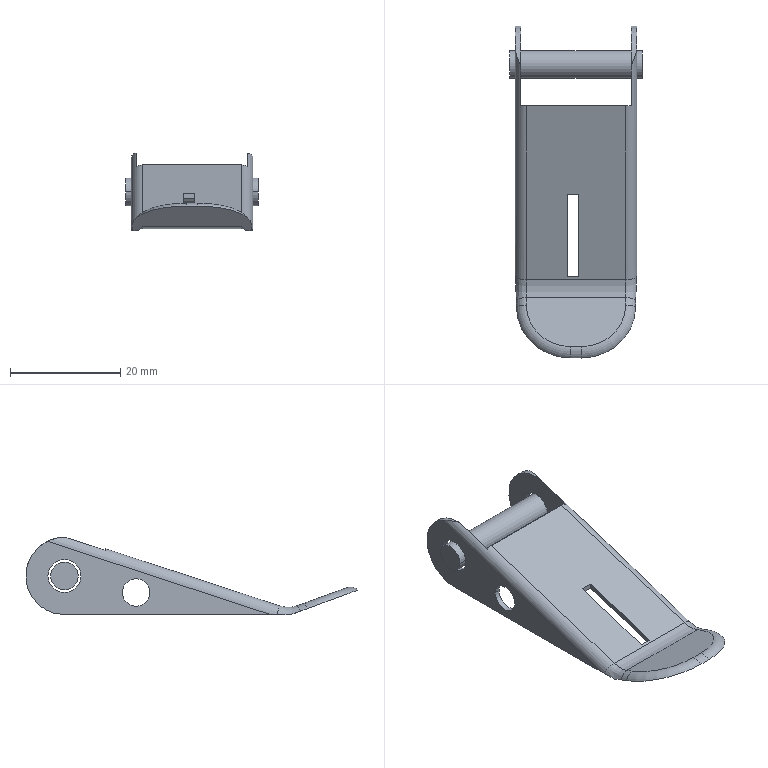Part | SolidWorks | features BaseBody 2 | 2 solids | 45 faces | box 24 x 60.185 x 14 mm | volume 1915 mm3 | cylinder 21 | plane 17 | torus 7 | commonest cylinder face diameters 5 x6 4 x5 6 x4 2 x2 14 x2 10 x1